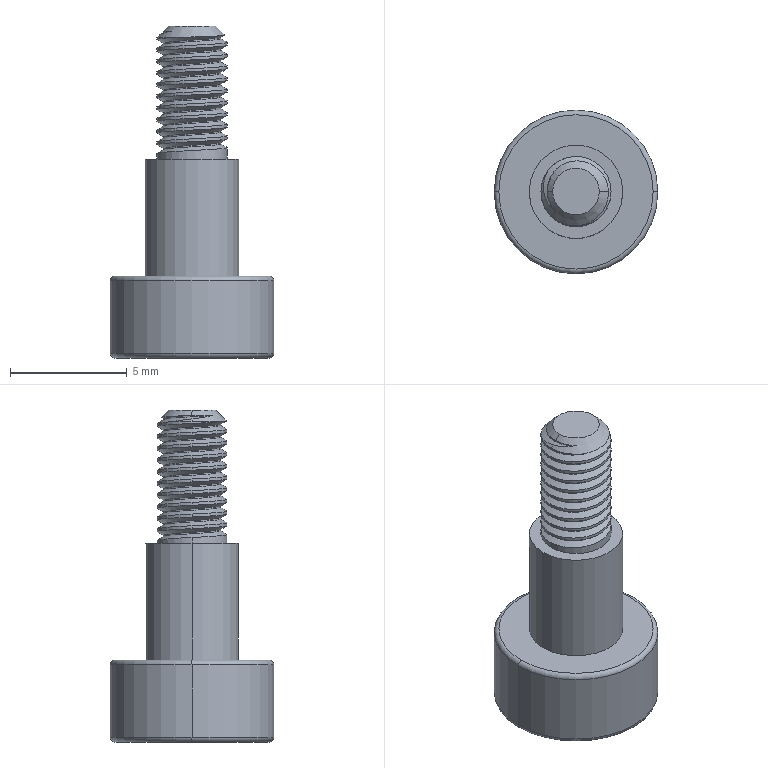Part | SolidWorks | features ICE 3, Chamfer 1, Extrusion 1, Fillet 1, SweepThread 1 | 1 solid | 50 faces | box 7 x 7 x 14.2 mm | volume 193.763 mm3 | cylinder 26 | plane 14 | torus 4 | cone 3 | spline 3 | commonest cylinder face diameters 3 x22 4 x2 7 x2